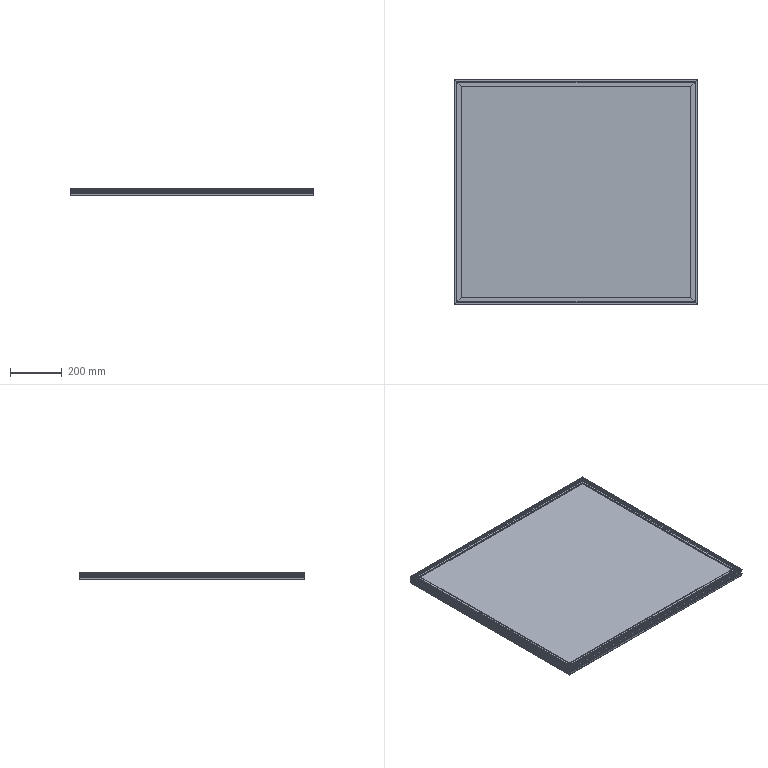Part | 5 solids | 272 faces | box 940 x 870 x 30 mm | volume 13230016 mm3 | plane 222 | cylinder 50 | commonest cylinder face diameters 0.4 x26 2 x16 1 x8